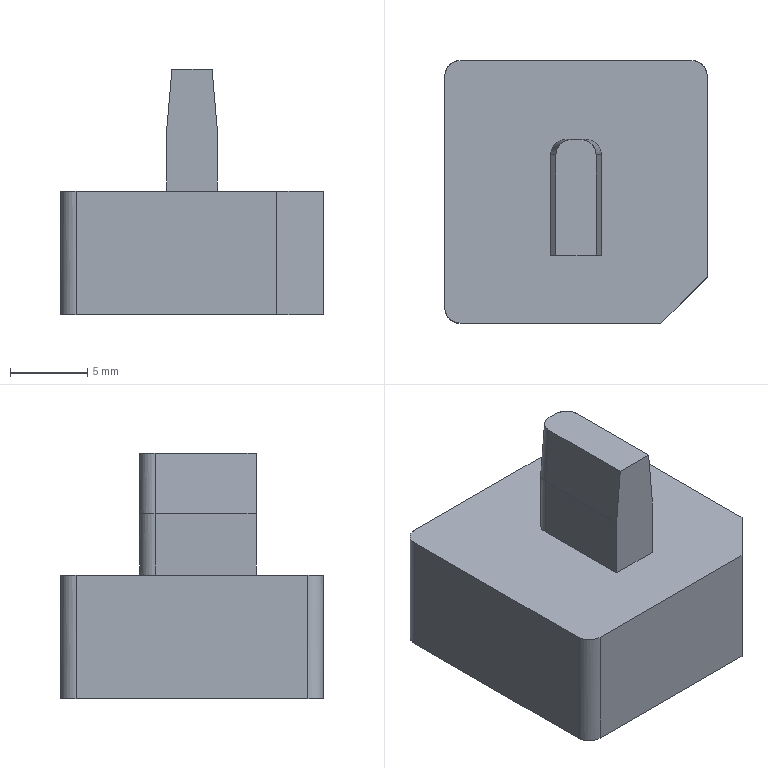NC program | PowerMill | posted with a generic post | part box 17 x 17 x 15.883 mm
Lines 2822 to 3515 of 37483:
N2919 M6
N2920 S8500 M03
N2921 G00 G90 X0.0 Y0.0
N2922 G43 Z11.804 H3
N2923
N2924 G05 P10000 R8
N2925 X-11.9584 Y-1.848
N2926 Z0.9329
N2927 G01 Z-0.2671 F360.0
N2928 X-6.6834 F600.0
N2929 X-2.6004 Y-1.5671
N2930 G03 X-0.6172 Y-3.4284 I1.9938 J0.1372
N2931 G01 X0.5417 Y-3.4345
N2932 G03 X2.5485 Y-1.3402 I0.0106 J1.9985
N2933 G01 X2.4342 Y1.0396
N2934 G03 X-1.4783 Y1.7132 I-2.031 J-0.0975
N2935 G01 X-2.4559 Y-0.6721
N2936 G03 X-2.6004 Y-1.5671 I1.8493 J-0.7578
N2937 G01 X-6.6834 Y-1.848
N2938 G00 Z11.804
N2939 G05 P0
N2940 (---------------)
N2941 ( END TOOLPATH : 精公基准台01-平坦面偏置-D10 )
N2942 (---------------)
N2943 ( START TOOLPATH : 精公基准台01-基准面偏置-D10 )
N2944 (---------------)
N2945 G00 X0.0 Y0.0 Z9.8056
N2946 G05 P10000 R8
N2947 X15.3207 Y-13.7546
N2948 Z-6.88
N2949 G01 Z-8.08 F360.0
N2950 X11.5907 Y-10.0247 F600.0
N2951 X7.0191 Y-0.8815
N2952 Y-4.15
N2953 X7.0117 Y-4.4316
N2954 X6.9896 Y-4.7124
N2955 X6.9528 Y-4.9916
N2956 X6.9015 Y-5.2686
N2957 X6.8357 Y-5.5424
N2958 X6.7558 Y-5.8125
N2959 X6.6617 Y-6.078
N2960 X6.5539 Y-6.3382
N2961 X6.4327 Y-6.5925
N2962 X6.2983 Y-6.84
N2963 X6.1511 Y-7.0802
N2964 X5.9916 Y-7.3123
N2965 G02 X5.6372 Y-7.7499 I-5.1269 J3.7895
N2966 G01 X5.4433 Y-7.9542
N2967 X5.239 Y-8.1481
N2968 X5.0248 Y-8.331
N2969 X4.8218 Y-8.4868
N2970 X4.6674 Y-8.5957
N2971 X4.5091 Y-8.6989
N2972 X4.3291 Y-8.8092
N2973 X4.0815 Y-8.9436
N2974 X3.8273 Y-9.0649
N2975 X3.5671 Y-9.1727
N2976 X3.3016 Y-9.2667
N2977 G02 X2.7576 Y-9.4124 I-1.9128 J6.0505
N2978 G01 X2.4807 Y-9.4638
N2979 X2.2014 Y-9.5005
N2980 X1.9206 Y-9.5226
N2981 X1.6391 Y-9.53
N2982 X-1.6391
N2983 X-1.9206 Y-9.5226
N2984 X-2.2014 Y-9.5005
N2985 X-2.4807 Y-9.4638
N2986 X-2.7576 Y-9.4124
N2987 X-3.0315 Y-9.3467
N2988 X-3.3016 Y-9.2667
N2989 X-3.5671 Y-9.1727
N2990 X-3.8273 Y-9.0649
N2991 G02 X-4.5692 Y-8.662 I2.3554 J5.2227
N2992 G01 X-4.8014 Y-8.5025
N2993 X-5.0248 Y-8.331
N2994 X-5.239 Y-8.1481
N2995 X-5.4433 Y-7.9542
N2996 G02 X-5.8201 Y-7.5357 I4.4958 J4.4268
N2997 G01 X-5.9916 Y-7.3123
N2998 X-6.1511 Y-7.0802
N2999 X-6.2983 Y-6.84
N3000 X-6.4327 Y-6.5925
N3001 X-6.5539 Y-6.3383
N3002 G02 X-6.7557 Y-5.8125 I5.6594 J2.474
N3003 G01 X-6.8357 Y-5.5425
N3004 X-6.9015 Y-5.2686
N3005 X-6.9528 Y-4.9916
N3006 X-6.9896 Y-4.7124
N3007 X-7.0117 Y-4.4316
N3008 X-7.0191 Y-4.15
N3009 Y2.3871
N3010 G02 X-6.8749 Y3.7347 I6.6782 J-0.0326
N3011 G01 X-6.8001 Y4.04
N3012 G02 X-6.4215 Y5.081 I6.163 J-1.6524
N3013 G01 X-6.3157 Y5.2981
N3014 G02 X-5.9459 Y5.9273 I6.3485 J-3.3091
N3015 G02 X-5.5386 Y6.4722 I5.7248 J-3.8538
N3016 G01 X-5.3074 Y6.7319
N3017 X-5.148 Y6.8997
N3018 X-4.8694 Y7.1603
N3019 X-4.6643 Y7.3358
N3020 X-4.3694 Y7.5603
N3021 G02 X-3.7016 Y7.9804 I3.5554 J-4.9112
N3022 G02 X-3.1957 Y8.2311 I2.9925 J-5.403
N3023 G01 X-2.9702 Y8.3248
N3024 G02 X-2.168 Y8.5802 I2.5966 J-6.7689
N3025 G02 X-1.5817 Y8.6963 I1.9474 J-8.2937
N3026 G01 X-1.3506 Y8.7267
N3027 G02 X-0.6352 Y8.7671 I0.7968 J-7.7501
N3028 G01 X0.6352
N3029 G02 X1.6508 Y8.6856 I-0.0488 J-6.9765
N3030 G02 X2.4698 Y8.4979 I-1.2474 J-7.3234
N3031 G01 X2.8126 Y8.3827
N3032 X3.0529 Y8.2918
N3033 X3.4003 Y8.1364
N3034 X3.6349 Y8.0188
N3035 X3.8635 Y7.8899
N3036 G02 X4.6325 Y7.3603 I-3.2162 J-5.4921
N3037 G01 X4.8706 Y7.1594
N3038 G02 X5.4419 Y6.5824 I-3.8996 J-4.433
N3039 G02 X5.7662 Y6.1826 I-4.4767 J-3.9629
N3040 G02 X6.1332 Y5.6273 I-6.2374 J-4.5215
N3041 G02 X6.5808 Y4.7095 I-5.7229 J-3.3586
N3042 G02 X6.7831 Y4.1043 I-8.0537 J-3.0294
N3043 G02 X6.9907 Y2.9772 I-6.4634 J-1.773
N3044 G02 X7.0191 Y2.3871 I-7.1051 J-0.637
N3045 G01 Y-0.8815
N3046 G00 Z9.8056
N3047 G05 P0
N3048 (---------------)
N3049 ( END TOOLPATH : 精公基准台01-基准面偏置-D10 )
N3050 (---------------)
N3051 ( START TOOLPATH : 精公基准台01-基准台侧光-D10 )
N3052 (---------------)
N3053 G00 X0.0 Y0.0 Z9.8056
N3054 G05 P10000 R8
N3055 X13.4804 Y-14.7749
N3056 Z-14.78
N3057 G01 Z-15.98 F360.0
N3058 G03 X9.9449 Y-11.2393 I-1.7677 J1.7678 F600.0
N3059 G01 X9.1141 Y-12.0701
N3060 X9.1135 Y-12.0707
N3061 X9.1128 Y-12.0714
N3062 X8.9074 Y-12.2678
N3063 X8.906 Y-12.269
N3064 X8.9046 Y-12.2703
N3065 X8.7671 Y-12.39
N3066 X8.7659 Y-12.3911
N3067 X8.7646 Y-12.3921
N3068 X8.5859 Y-12.5352
N3069 X8.5843 Y-12.5365
N3070 X8.5826 Y-12.5378
N3071 X8.3417 Y-12.7108
N3072 X8.3404 Y-12.7117
N3073 X8.3391 Y-12.7126
N3074 X8.2639 Y-12.7623
N3075 X8.2624 Y-12.7633
N3076 X8.2608 Y-12.7643
N3077 X7.9447 Y-12.953
N3078 X7.9428 Y-12.9541
N3079 X7.9409 Y-12.9551
N3080 X7.7936 Y-13.0328
N3081 X7.7923 Y-13.0334
N3082 X7.791 Y-13.034
N3083 X7.6223 Y-13.1154
N3084 X7.6203 Y-13.1163
N3085 X7.6184 Y-13.1172
N3086 X7.3022 Y-13.2495
N3087 X7.2998 Y-13.2505
N3088 X7.2973 Y-13.2514
N3089 X6.9989 Y-13.3538
N3090 X6.9964 Y-13.3546
N3091 X6.9939 Y-13.3553
N3092 X6.66 Y-13.4457
N3093 X6.6574 Y-13.4464
N3094 X6.6548 Y-13.447
N3095 X6.3386 Y-13.5103
N3096 X6.3361 Y-13.5107
N3097 X6.3336 Y-13.5111
N3098 X6.0174 Y-13.5535
N3099 X6.0149 Y-13.5538
N3100 X6.0124 Y-13.5541
N3101 X5.6962 Y-13.5762
N3102 X5.6939 Y-13.5763
N3103 X5.6915 Y-13.5764
N3104 X5.3754 Y-13.58
N3105 X5.3749
N3106 X5.3745
N3107 X-7.5875 Y-13.5792
N3108 X-7.5891
N3109 X-7.5907
N3110 X-7.9069 Y-13.5663
N3111 X-7.909 Y-13.5662
N3112 X-7.9111 Y-13.5661
N3113 X-8.2273 Y-13.5363
N3114 X-8.2294 Y-13.536
N3115 X-8.2315 Y-13.5357
N3116 X-8.5476 Y-13.489
N3117 X-8.5498 Y-13.4887
N3118 X-8.5519 Y-13.4883
N3119 X-8.868 Y-13.424
N3120 X-8.87 Y-13.4236
N3121 X-8.8719 Y-13.4232
N3122 X-9.1361 Y-13.3556
N3123 X-9.1383 Y-13.3551
N3124 X-9.1404 Y-13.3544
N3125 X-9.5084 Y-13.2385
N3126 X-9.5107 Y-13.2377
N3127 X-9.5129 Y-13.2369
N3128 X-9.8291 Y-13.1162
N3129 X-9.8308 Y-13.1155
N3130 X-9.8324 Y-13.1148
N3131 X-10.0152 Y-13.0353
N3132 X-10.0162 Y-13.0349
N3133 X-10.0173 Y-13.0344
N3134 X-10.1507 Y-12.9716
N3135 X-10.1522 Y-12.9708
N3136 X-10.1537 Y-12.9701
N3137 X-10.4698 Y-12.8052
N3138 X-10.4714 Y-12.8044
N3139 X-10.4729 Y-12.8035
N3140 X-10.6255 Y-12.715
N3141 X-10.6266 Y-12.7144
N3142 X-10.6277 Y-12.7137
N3143 X-10.7912 Y-12.612
N3144 X-10.7928 Y-12.611
N3145 X-10.7943 Y-12.6099
N3146 X-11.1054 Y-12.3956
N3147 X-11.1076 Y-12.394
N3148 X-11.1097 Y-12.3924
N3149 X-11.4309 Y-12.1383
N3150 X-11.4322 Y-12.1372
N3151 X-11.4335 Y-12.1362
N3152 X-11.5055 Y-12.0741
N3153 X-11.5065 Y-12.0732
N3154 X-11.5076 Y-12.0722
N3155 X-11.7518 Y-11.846
N3156 X-11.7529 Y-11.845
N3157 X-11.754 Y-11.8439
N3158 X-11.8439 Y-11.754
N3159 X-11.845 Y-11.7529
N3160 X-11.846 Y-11.7517
N3161 X-12.0722 Y-11.5074
N3162 X-12.0733 Y-11.5062
N3163 X-12.0744 Y-11.505
N3164 X-12.1357 Y-11.4332
N3165 X-12.1367 Y-11.4321
N3166 X-12.1376 Y-11.431
N3167 X-12.3886 Y-11.1148
N3168 X-12.3902 Y-11.1127
N3169 X-12.3918 Y-11.1105
N3170 X-12.6097 Y-10.7944
N3171 X-12.6108 Y-10.7928
N3172 X-12.6118 Y-10.7913
N3173 X-12.7137 Y-10.6278
N3174 X-12.7144 Y-10.6266
N3175 X-12.715 Y-10.6255
N3176 X-12.8035 Y-10.4729
N3177 X-12.8043 Y-10.4714
N3178 X-12.8052 Y-10.4698
N3179 X-12.9703 Y-10.1537
N3180 X-12.9713 Y-10.1516
N3181 X-12.9723 Y-10.1495
N3182 X-13.1144 Y-9.8333
N3183 X-13.1153 Y-9.8312
N3184 X-13.1162 Y-9.8291
N3185 X-13.237 Y-9.5129
N3186 X-13.2378 Y-9.5108
N3187 X-13.2385 Y-9.5087
N3188 X-13.3396 Y-9.1926
N3189 X-13.3402 Y-9.1905
N3190 X-13.3408 Y-9.1884
N3191 X-13.4231 Y-8.8722
N3192 X-13.4236 Y-8.87
N3193 X-13.4241 Y-8.8678
N3194 X-13.4876 Y-8.5517
N3195 X-13.488 Y-8.5497
N3196 X-13.4883 Y-8.5478
N3197 X-13.5357 Y-8.2317
N3198 X-13.536 Y-8.2294
N3199 X-13.5363 Y-8.2271
N3200 X-13.5653 Y-7.911
N3201 X-13.5655 Y-7.909
N3202 X-13.5656 Y-7.9071
N3203 X-13.5792 Y-7.5909
N3204 Y-7.5892
N3205 Y-7.5875
N3206 Y0.0
N3207 Y7.5875
N3208 Y7.5891
N3209 Y7.5907
N3210 X-13.5663 Y7.9069
N3211 X-13.5662 Y7.909
N3212 X-13.5661 Y7.9111
N3213 X-13.5363 Y8.2273
N3214 X-13.536 Y8.2294
N3215 X-13.5357 Y8.2315
N3216 X-13.489 Y8.5476
N3217 X-13.4887 Y8.5498
N3218 X-13.4883 Y8.5519
N3219 X-13.424 Y8.868
N3220 X-13.4236 Y8.87
N3221 X-13.4232 Y8.8719
N3222 X-13.3556 Y9.1361
N3223 X-13.3551 Y9.1383
N3224 X-13.3544 Y9.1404
N3225 X-13.2385 Y9.5084
N3226 X-13.2377 Y9.5107
N3227 X-13.2369 Y9.5129
N3228 X-13.1162 Y9.8291
N3229 X-13.1155 Y9.8308
N3230 X-13.1148 Y9.8324
N3231 X-13.0353 Y10.0152
N3232 X-13.0349 Y10.0162
N3233 X-13.0344 Y10.0173
N3234 X-12.9716 Y10.1507
N3235 X-12.9708 Y10.1522
N3236 X-12.9701 Y10.1537
N3237 X-12.8052 Y10.4698
N3238 X-12.8044 Y10.4714
N3239 X-12.8035 Y10.4729
N3240 X-12.715 Y10.6255
N3241 X-12.7144 Y10.6266
N3242 X-12.7137 Y10.6277
N3243 X-12.612 Y10.7912
N3244 X-12.611 Y10.7928
N3245 X-12.6099 Y10.7943
N3246 X-12.3956 Y11.1054
N3247 X-12.394 Y11.1076
N3248 X-12.3924 Y11.1097
N3249 X-12.1383 Y11.4309
N3250 X-12.1372 Y11.4322
N3251 X-12.1362 Y11.4335
N3252 X-12.0741 Y11.5055
N3253 X-12.0732 Y11.5065
N3254 X-12.0722 Y11.5076
N3255 X-11.846 Y11.7518
N3256 X-11.845 Y11.7529
N3257 X-11.8439 Y11.754
N3258 X-11.754 Y11.8439
N3259 X-11.7529 Y11.845
N3260 X-11.7517 Y11.846
N3261 X-11.5074 Y12.0722
N3262 X-11.5062 Y12.0733
N3263 X-11.505 Y12.0744
N3264 X-11.4332 Y12.1357
N3265 X-11.4321 Y12.1367
N3266 X-11.431 Y12.1376
N3267 X-11.1148 Y12.3886
N3268 X-11.1127 Y12.3902
N3269 X-11.1105 Y12.3918
N3270 X-10.7944 Y12.6097
N3271 X-10.7928 Y12.6108
N3272 X-10.7913 Y12.6118
N3273 X-10.6278 Y12.7137
N3274 X-10.6266 Y12.7144
N3275 X-10.6255 Y12.715
N3276 X-10.4729 Y12.8035
N3277 X-10.4714 Y12.8043
N3278 X-10.4698 Y12.8052
N3279 X-10.1537 Y12.9703
N3280 X-10.1516 Y12.9713
N3281 X-10.1495 Y12.9723
N3282 X-9.8333 Y13.1144
N3283 X-9.8312 Y13.1153
N3284 X-9.8291 Y13.1162
N3285 X-9.5129 Y13.237
N3286 X-9.5108 Y13.2378
N3287 X-9.5087 Y13.2385
N3288 X-9.1926 Y13.3396
N3289 X-9.1905 Y13.3402
N3290 X-9.1884 Y13.3408
N3291 X-8.8722 Y13.4231
N3292 X-8.87 Y13.4236
N3293 X-8.8678 Y13.4241
N3294 X-8.5517 Y13.4876
N3295 X-8.5497 Y13.488
N3296 X-8.5478 Y13.4883
N3297 X-8.2317 Y13.5357
N3298 X-8.2294 Y13.536
N3299 X-8.2271 Y13.5363
N3300 X-7.911 Y13.5653
N3301 X-7.909 Y13.5655
N3302 X-7.9071 Y13.5656
N3303 X-7.5909 Y13.5792
N3304 X-7.5892
N3305 X-7.5875
N3306 X7.5875
N3307 X7.5891
N3308 X7.5907
N3309 X7.9069 Y13.5663
N3310 X7.909 Y13.5662
N3311 X7.9111 Y13.5661
N3312 X8.2273 Y13.5363
N3313 X8.2294 Y13.536
N3314 X8.2315 Y13.5357
N3315 X8.5476 Y13.489
N3316 X8.5498 Y13.4887
N3317 X8.5519 Y13.4883
N3318 X8.868 Y13.424
N3319 X8.87 Y13.4236
N3320 X8.8719 Y13.4232
N3321 X9.1361 Y13.3556
N3322 X9.1383 Y13.3551
N3323 X9.1404 Y13.3544
N3324 X9.5084 Y13.2385
N3325 X9.5107 Y13.2377
N3326 X9.5129 Y13.2369
N3327 X9.8291 Y13.1162
N3328 X9.8308 Y13.1155
N3329 X9.8324 Y13.1148
N3330 X10.0152 Y13.0353
N3331 X10.0162 Y13.0349
N3332 X10.0173 Y13.0344
N3333 X10.1507 Y12.9716
N3334 X10.1522 Y12.9708
N3335 X10.1537 Y12.9701
N3336 X10.4698 Y12.8052
N3337 X10.4714 Y12.8044
N3338 X10.4729 Y12.8035
N3339 X10.6255 Y12.715
N3340 X10.6266 Y12.7144
N3341 X10.6277 Y12.7137
N3342 X10.7912 Y12.612
N3343 X10.7928 Y12.611
N3344 X10.7943 Y12.6099
N3345 X11.1054 Y12.3956
N3346 X11.1076 Y12.394
N3347 X11.1097 Y12.3924
N3348 X11.4309 Y12.1383
N3349 X11.4322 Y12.1372
N3350 X11.4335 Y12.1362
N3351 X11.5055 Y12.0741
N3352 X11.5065 Y12.0732
N3353 X11.5076 Y12.0722
N3354 X11.7518 Y11.846
N3355 X11.7529 Y11.845
N3356 X11.754 Y11.8439
N3357 X11.8439 Y11.754
N3358 X11.845 Y11.7529
N3359 X11.846 Y11.7517
N3360 X12.0722 Y11.5074
N3361 X12.0733 Y11.5062
N3362 X12.0744 Y11.505
N3363 X12.1357 Y11.4332
N3364 X12.1367 Y11.4321
N3365 X12.1376 Y11.431
N3366 X12.3886 Y11.1148
N3367 X12.3902 Y11.1127
N3368 X12.3918 Y11.1105
N3369 X12.6097 Y10.7944
N3370 X12.6108 Y10.7928
N3371 X12.6118 Y10.7913
N3372 X12.7137 Y10.6278
N3373 X12.7144 Y10.6266
N3374 X12.715 Y10.6255
N3375 X12.8035 Y10.4729
N3376 X12.8043 Y10.4714
N3377 X12.8052 Y10.4698
N3378 X12.9703 Y10.1537
N3379 X12.9713 Y10.1516
N3380 X12.9723 Y10.1495
N3381 X13.1144 Y9.8333
N3382 X13.1153 Y9.8312
N3383 X13.1162 Y9.8291
N3384 X13.237 Y9.5129
N3385 X13.2378 Y9.5108
N3386 X13.2385 Y9.5087
N3387 X13.3396 Y9.1926
N3388 X13.3402 Y9.1905
N3389 X13.3408 Y9.1884
N3390 X13.4231 Y8.8722
N3391 X13.4236 Y8.87
N3392 X13.4241 Y8.8678
N3393 X13.4876 Y8.5517
N3394 X13.488 Y8.5497
N3395 X13.4883 Y8.5478
N3396 X13.5357 Y8.2317
N3397 X13.536 Y8.2294
N3398 X13.5363 Y8.2271
N3399 X13.5653 Y7.911
N3400 X13.5655 Y7.909
N3401 X13.5656 Y7.9071
N3402 X13.5792 Y7.5909
N3403 Y7.5892
N3404 Y7.5875
N3405 X13.58 Y-5.3745
N3406 Y-5.3749
N3407 Y-5.3754
N3408 X13.5764 Y-5.6915
N3409 X13.5763 Y-5.6939
N3410 X13.5762 Y-5.6962
N3411 X13.5541 Y-6.0124
N3412 X13.5538 Y-6.0149
N3413 X13.5535 Y-6.0174
N3414 X13.5111 Y-6.3336
N3415 X13.5107 Y-6.3361
N3416 X13.5103 Y-6.3386
N3417 X13.447 Y-6.6548
N3418 X13.4464 Y-6.6573
N3419 X13.4458 Y-6.6598
N3420 X13.3608 Y-6.976
N3421 X13.3601 Y-6.9785
N3422 X13.3593 Y-6.981
N3423 X13.2514 Y-7.2972
N3424 X13.2505 Y-7.2997
N3425 X13.2495 Y-7.3022
N3426 X13.1172 Y-7.6184
N3427 X13.1163 Y-7.6203
N3428 X13.1154 Y-7.6223
N3429 X13.034 Y-7.791
N3430 X13.0334 Y-7.7923
N3431 X13.0328 Y-7.7936
N3432 X12.9551 Y-7.9409
N3433 X12.9541 Y-7.9428
N3434 X12.953 Y-7.9447
N3435 X12.7643 Y-8.2608
N3436 X12.7633 Y-8.2624
N3437 X12.7623 Y-8.2639
N3438 X12.7126 Y-8.3391
N3439 X12.7117 Y-8.3404
N3440 X12.7108 Y-8.3417
N3441 X12.5378 Y-8.5826
N3442 X12.5365 Y-8.5843
N3443 X12.5352 Y-8.5859
N3444 X12.3921 Y-8.7646
N3445 X12.3911 Y-8.7659
N3446 X12.39 Y-8.7671
N3447 X12.2703 Y-8.9046
N3448 X12.269 Y-8.906
N3449 X12.2678 Y-8.9074
N3450 X12.0714 Y-9.1128
N3451 X12.0707 Y-9.1135
N3452 X12.0701 Y-9.1141
N3453 X9.9449 Y-11.2393
N3454 G03 X13.4804 Y-14.7749 I1.7678 J-1.7678
N3455 G01 X13.4289 Y-14.7132
N3456 G03 X9.8934 Y-11.1777 I-1.7677 J1.7678
N3457 G01 X9.0575 Y-12.0135
N3458 X8.8521 Y-12.2099
N3459 X8.7146 Y-12.3297
N3460 X8.5359 Y-12.4728
N3461 X8.295 Y-12.6458
N3462 X8.2198 Y-12.6956
N3463 X7.9036 Y-12.8844
N3464 X7.7563 Y-12.962
N3465 X7.5875 Y-13.0434
N3466 X7.2714 Y-13.1757
N3467 X6.973 Y-13.2781
N3468 X6.6391 Y-13.3685
N3469 X6.3229 Y-13.4318
N3470 X6.0068 Y-13.4743
N3471 X5.6906 Y-13.4964
N3472 X5.3745 Y-13.5
N3473 X-7.2714
N3474 X-7.5875 Y-13.4992
N3475 X-7.9036 Y-13.4864
N3476 X-8.2198 Y-13.4566
N3477 X-8.5359 Y-13.4099
N3478 X-8.8521 Y-13.3456
N3479 X-9.1163 Y-13.2781
N3480 X-9.4844 Y-13.1622
N3481 X-9.8005 Y-13.0415
N3482 X-9.9832 Y-12.962
N3483 X-10.1167 Y-12.8992
N3484 X-10.4328 Y-12.7343
N3485 X-10.5854 Y-12.6458
N3486 X-10.749 Y-12.544
N3487 X-11.06 Y-12.3297
N3488 X-11.3812 Y-12.0756
N3489 X-11.4532 Y-12.0135
N3490 X-11.6974 Y-11.7873
N3491 X-11.7873 Y-11.6974
N3492 X-12.0135 Y-11.4531
N3493 X-12.0749 Y-11.3812
N3494 X-12.3259 Y-11.0651
N3495 X-12.5439 Y-10.749
N3496 X-12.6458 Y-10.5854
N3497 X-12.7343 Y-10.4328
N3498 X-12.8994 Y-10.1167
N3499 X-13.0415 Y-9.8005
N3500 X-13.1623 Y-9.4844
N3501 X-13.2634 Y-9.1682
N3502 X-13.3457 Y-8.8521
N3503 X-13.4092 Y-8.5359
N3504 X-13.4566 Y-8.2198
N3505 X-13.4857 Y-7.9036
N3506 X-13.4992 Y-7.5875
N3507 X-13.5 Y-7.2714
N3508 Y0.0
N3509 Y7.2714
N3510 X-13.4992 Y7.5875
N3511 X-13.4864 Y7.9036
N3512 X-13.4566 Y8.2198
N3513 X-13.4099 Y8.5359
N3514 X-13.3456 Y8.8521
N3515 X-13.2781 Y9.1163
N3516 X-13.1622 Y9.4844
N3517 X-13.0415 Y9.8005
N3518 X-12.962 Y9.9832
N3519 X-12.8992 Y10.1167
N3520 X-12.7343 Y10.4328
N3521 X-12.6458 Y10.5854
N3522 X-12.544 Y10.749
N3523 X-12.3297 Y11.06
N3524 X-12.0756 Y11.3812
N3525 X-12.0135 Y11.4532
N3526 X-11.7873 Y11.6974
N3527 X-11.6974 Y11.7873
N3528 X-11.4531 Y12.0135
N3529 X-11.3812 Y12.0749
N3530 X-11.0651 Y12.3259
N3531 X-10.749 Y12.5439
N3532 X-10.5854 Y12.6458
N3533 X-10.4328 Y12.7343
N3534 X-10.1167 Y12.8994
N3535 X-9.8005 Y13.0415
N3536 X-9.4844 Y13.1623
N3537 X-9.1682 Y13.2634
N3538 X-8.8521 Y13.3457
N3539 X-8.5359 Y13.4092
N3540 X-8.2198 Y13.4566
N3541 X-7.9036 Y13.4857
N3542 X-7.5875 Y13.4992
N3543 X-7.2714 Y13.5
N3544 X7.2714
N3545 X7.5875 Y13.4992
N3546 X7.9036 Y13.4864
N3547 X8.2198 Y13.4566
N3548 X8.5359 Y13.4099
N3549 X8.8521 Y13.3456
N3550 X9.1163 Y13.2781
N3551 X9.4844 Y13.1622
N3552 X9.8005 Y13.0415
N3553 X9.9832 Y12.962
N3554 X10.1167 Y12.8992
N3555 X10.4328 Y12.7343
N3556 X10.5854 Y12.6458
N3557 X10.749 Y12.544
N3558 X11.06 Y12.3297
N3559 X11.3812 Y12.0756
N3560 X11.4532 Y12.0135
N3561 X11.6974 Y11.7873
N3562 X11.7873 Y11.6974
N3563 X12.0135 Y11.4531
N3564 X12.0749 Y11.3812
N3565 X12.3259 Y11.0651
N3566 X12.5439 Y10.749
N3567 X12.6458 Y10.5854
N3568 X12.7343 Y10.4328
N3569 X12.8994 Y10.1167
N3570 X13.0415 Y9.8005
N3571 X13.1623 Y9.4844
N3572 X13.2634 Y9.1682
N3573 X13.3457 Y8.8521
N3574 X13.4092 Y8.5359
N3575 X13.4566 Y8.2198
N3576 X13.4857 Y7.9036
N3577 X13.4992 Y7.5875
N3578 X13.5 Y7.2714
N3579 Y-5.3745
N3580 X13.4964 Y-5.6906
N3581 X13.4743 Y-6.0068
N3582 X13.4318 Y-6.3229
N3583 X13.3685 Y-6.6391
N3584 X13.2836 Y-6.9552
N3585 X13.1757 Y-7.2714
N3586 X13.0434 Y-7.5875
N3587 X12.962 Y-7.7563
N3588 X12.8844 Y-7.9036
N3589 X12.6956 Y-8.2198
N3590 X12.6458 Y-8.295
N3591 X12.4728 Y-8.5359
N3592 X12.3297 Y-8.7146
N3593 X12.2099 Y-8.8521
N3594 X12.0135 Y-9.0575
N3595 X9.8934 Y-11.1777
N3596 G03 X13.4289 Y-14.7132 I1.7678 J-1.7677
N3597 G00 Z9.8056
N3598 G05 P0
N3599 (---------------)
N3600 ( END TOOLPATH : 精公基准台01-基准台侧光-D10 )
N3601 (---------------)
N3602
N3603 M05
N3604 G53 Z0.0
N3605 (---------------)
N3606 ( START TOOLPATH : 精公精光01-等高-D4 )
N3607 (---------------)
N3608 ( TOOL NO.    :14 )
N3609 ( TOOL TYPE   : ENDMILL)
N3610 ( TOOL ID     : D4_1_1)
N3611 ( TOOL DIA    : 4.0 LENGTH 63.04)
N3612 T14